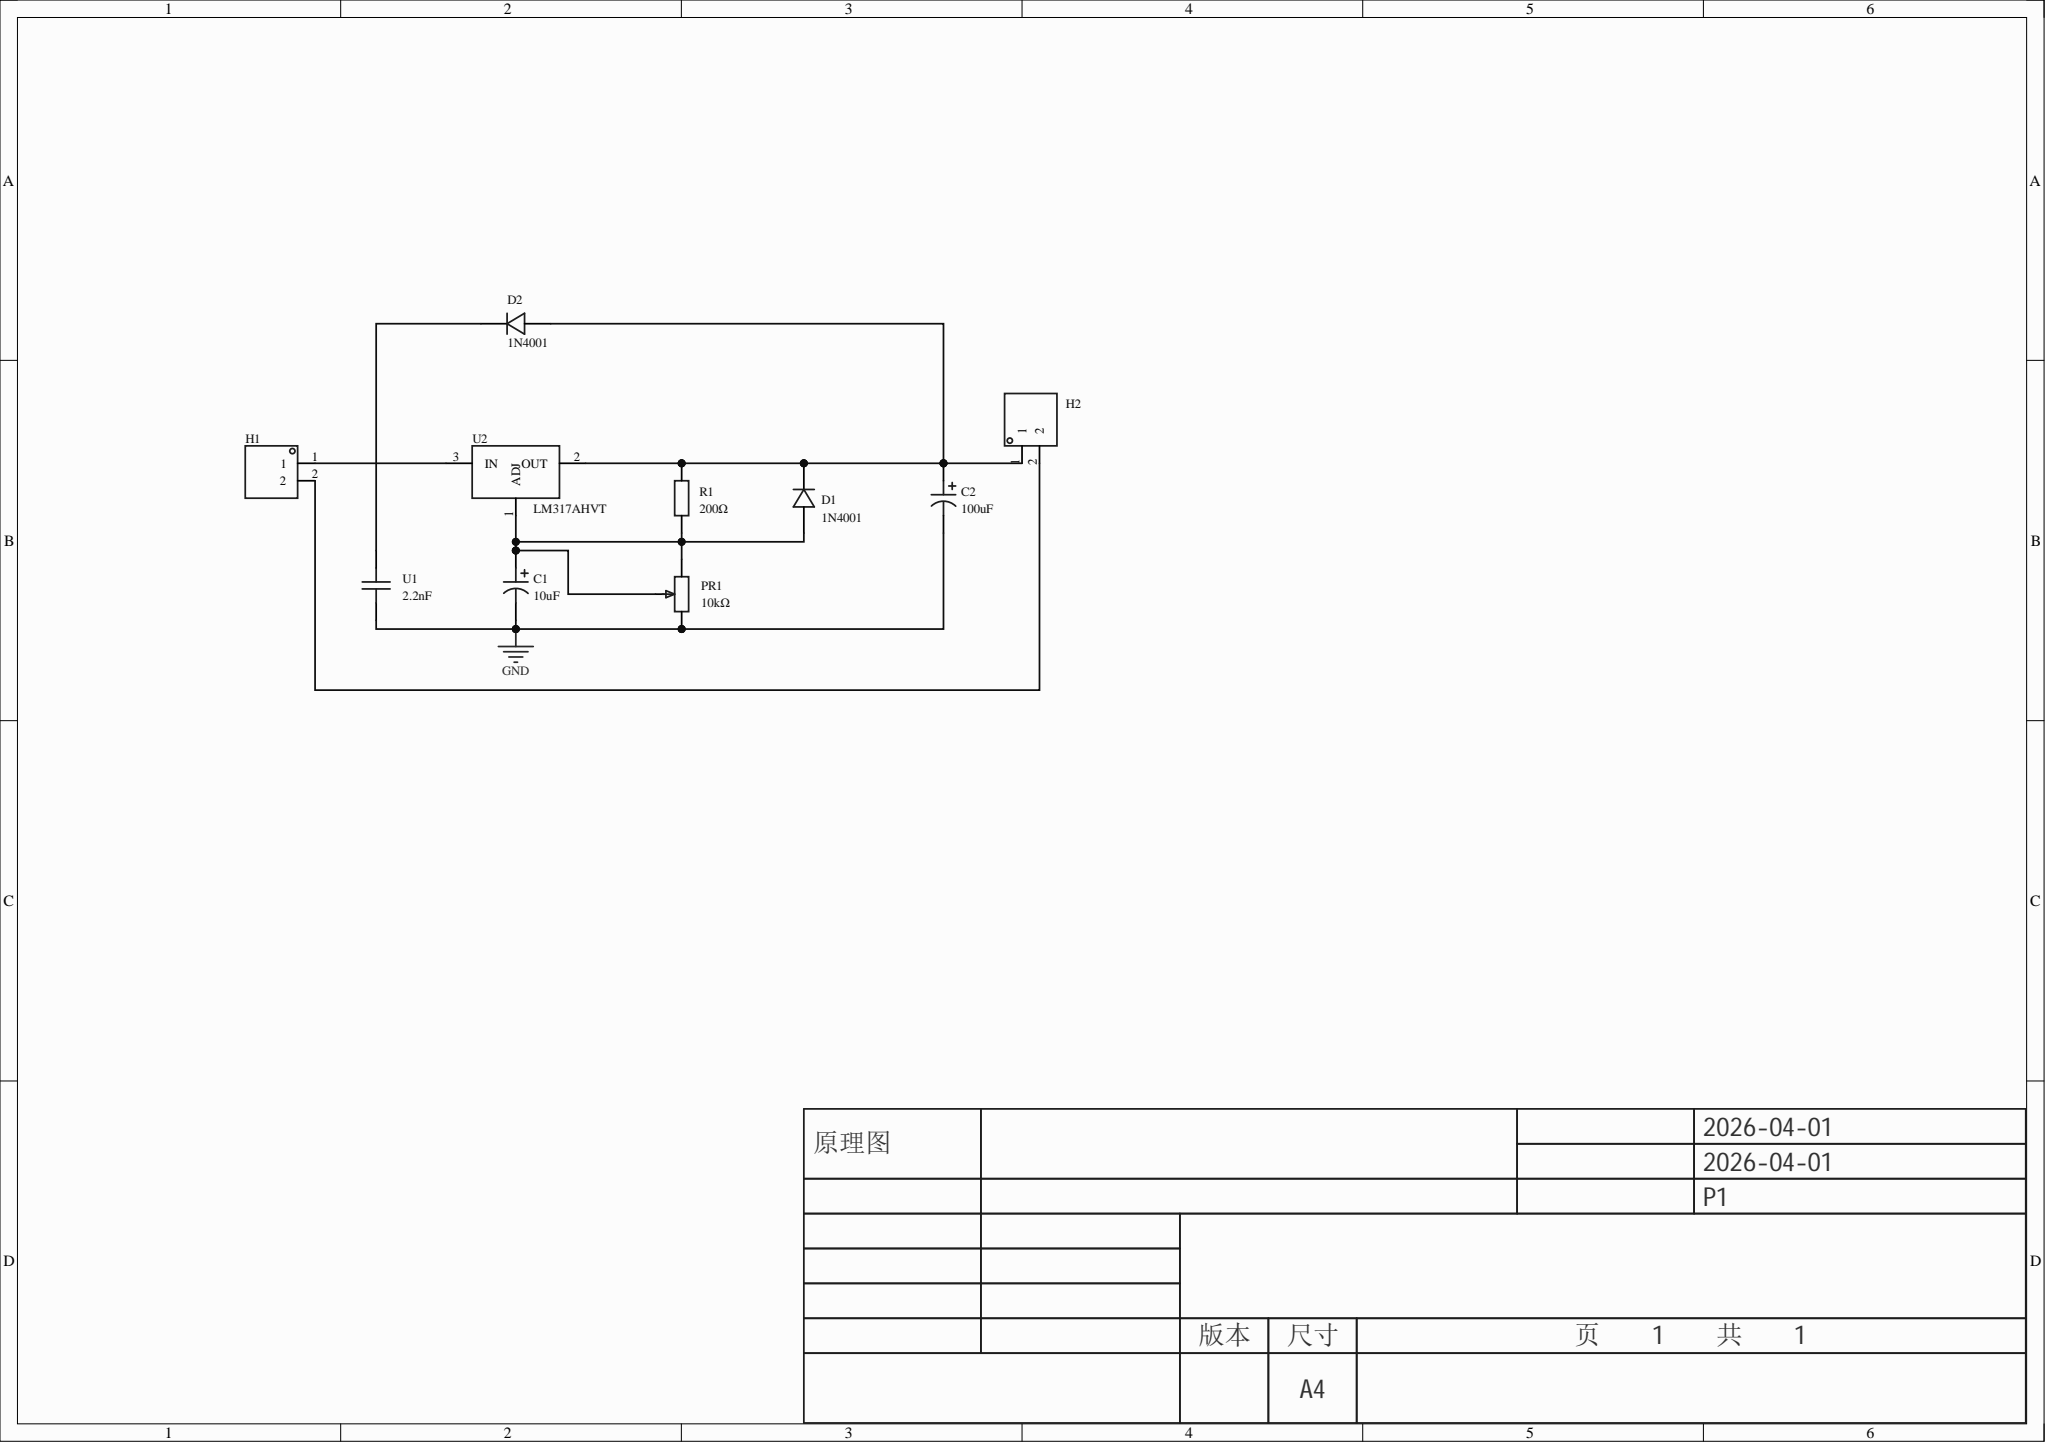Circuit board | Altium Designer | 10 parts | 6 nets
Bill of materials:
Comment,Description,Designator,Footprint,LibRef,Quantity
"10uF","","C1","CAP-TH_BD5.0-P2.00-D0.8-FD-10UF50VC110GL","10UF50VC110GL","1"
"100uF","","C2","CAP-TH_BD8.0-P3.50-D0.6-FD_1","100uF","1"
"1N4001","","D1, D2","DO-41_BD2.4-L4.7-P8.70-D0.8-RD","1N4001E-E3/73","2"
"","","H1, H2","HDR-TH_2P-P2.54-V-M-1","HDR-M_2.54_1x2P","2"
"10kΩ","","PR1","R_3296","R_3296","1"
"200Ω","","R1","Res_1/8W","Res_AXIAL-1/8W","1"
"2.2nF","","U1","CAP-TH_L5.0-W2.5-P5.00-D1.0","100nF","1"
"LM317AHVT","","U2","TO-220-3_L10.0-W4.5-P2.54-L","LM317AHVT","1"
Netlist (Protel format):
[
C1
CAP-TH_BD5.0-P2.00-D0.8-FD-10UF50VC110GL
10uF



]
[
C2
CAP-TH_BD8.0-P3.50-D0.6-FD_1
100uF



]
[
D1
DO-41_BD2.4-L4.7-P8.70-D0.8-RD
1N4001



]
[
D2
DO-41_BD2.4-L4.7-P8.70-D0.8-RD
1N4001



]
[
H1
HDR-TH_2P-P2.54-V-M-1




]
[
H2
HDR-TH_2P-P2.54-V-M-1




]
[
PR1
R_3296
10kΩ



]
[
R1
Res_1/8W
200Ω



]
[
U1
CAP-TH_L5.0-W2.5-P5.00-D1.0
2.2nF



]
[
U2
TO-220-3_L10.0-W4.5-P2.54-L
LM317AHVT



]
(
NetH1_2
H1-2
H2-2
)
(
NetH1_1
H1-1
U2-3
)
(
NetD2_1
D2-1
U1-1
)
(
NetC2_1
C2-1
D1-1
D2-2
H2-1
R1-2
U2-2
)
(
NetC1_1
C1-1
D1-2
PR1-1
PR1-2
R1-1
U2-1
)
(
GND
C1-2
C2-2
PR1-3
U1-2
)